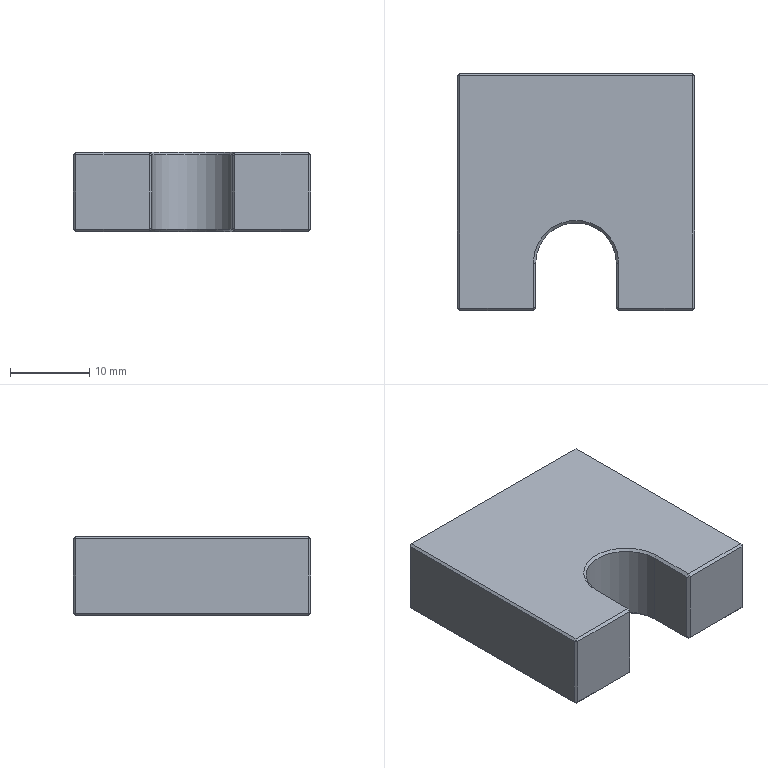Part | SolidWorks | features Chamfer 2, Extrusion 1, HoleWzd 1, ICE 1 | 1 solid | 52 faces | box 30 x 30 x 10 mm | volume 7510 mm3 | plane 41 | cone 6 | cylinder 5 | commonest cylinder face diameters 4.2 x4 10.2 x1
STEP:
#1=CARTESIAN_POINT('',(10.,-1.,2.9));
#2=VERTEX_POINT('',#1);
#3=CARTESIAN_POINT('',(10.,-1.,7.1));
#4=VERTEX_POINT('',#3);
#5=CARTESIAN_POINT('',(10.,-1.,5.));
#6=DIRECTION('',(0.,1.,0.));
#7=DIRECTION('',(0.,0.,1.));
#8=AXIS2_PLACEMENT_3D('',#5,#6,#7);
#9=CIRCLE('',#8,2.1);
#10=EDGE_CURVE('',#2,#4,#9,.T.);
#11=ORIENTED_EDGE('',*,*,#10,.F.);
#12=CARTESIAN_POINT('',(10.,15.,2.9));
#13=VERTEX_POINT('',#12);
#14=CARTESIAN_POINT('',(10.,15.,2.9));
#15=DIRECTION('',(0.,1.,0.));
#16=VECTOR('',#15,1000.);
#17=LINE('',#14,#16);
#18=EDGE_CURVE('',#2,#13,#17,.T.);
#19=ORIENTED_EDGE('',*,*,#18,.T.);
#20=CARTESIAN_POINT('',(10.,15.,7.1));
#21=VERTEX_POINT('',#20);
#22=CARTESIAN_POINT('',(10.,15.,5.));
#23=DIRECTION('',(0.,1.,0.));
#24=DIRECTION('',(0.,0.,1.));
#25=AXIS2_PLACEMENT_3D('',#22,#23,#24);
#26=CIRCLE('',#25,2.1);
#27=EDGE_CURVE('',#13,#21,#26,.T.);
#28=ORIENTED_EDGE('',*,*,#27,.T.);
#29=CARTESIAN_POINT('',(10.,15.,7.1));
#30=DIRECTION('',(0.,1.,0.));
#31=VECTOR('',#30,1000.);
#32=LINE('',#29,#31);
#33=EDGE_CURVE('',#4,#21,#32,.T.);
#34=ORIENTED_EDGE('',*,*,#33,.F.);
#35=EDGE_LOOP('',(#11,#19,#28,#34));
#36=FACE_OUTER_BOUND('',#35,.T.);
#37=CARTESIAN_POINT('',(10.,15.,5.));
#38=DIRECTION('',(0.,1.,0.));
#39=DIRECTION('',(0.,0.,1.));
#40=AXIS2_PLACEMENT_3D('',#37,#38,#39);
#41=CYLINDRICAL_SURFACE('',#40,2.1);
#42=ADVANCED_FACE('',(#36),#41,.F.);
#43=CARTESIAN_POINT('',(10.,-2.262,5.));
#44=VERTEX_POINT('',#43);
#45=CARTESIAN_POINT('',(10.,-1.,7.1));
#46=DIRECTION('',(0.,0.515,0.8572));
#47=VECTOR('',#46,1000.);
#48=LINE('',#45,#47);
#49=EDGE_CURVE('',#44,#4,#48,.T.);
#50=ORIENTED_EDGE('',*,*,#49,.F.);
#51=CARTESIAN_POINT('',(10.,-1.,2.9));
#52=DIRECTION('',(0.,0.515,-0.8572));
#53=VECTOR('',#52,1000.);
#54=LINE('',#51,#53);
#55=EDGE_CURVE('',#44,#2,#54,.T.);
#56=ORIENTED_EDGE('',*,*,#55,.T.);
#57=ORIENTED_EDGE('',*,*,#10,.T.);
#58=EDGE_LOOP('',(#50,#56,#57));
#59=FACE_OUTER_BOUND('',#58,.T.);
#60=CARTESIAN_POINT('',(10.,-1.,5.));
#61=DIRECTION('',(0.,1.,0.));
#62=DIRECTION('',(0.,0.,1.));
#63=AXIS2_PLACEMENT_3D('',#60,#61,#62);
#64=CONICAL_SURFACE('',#63,2.1,1.03);
#65=ADVANCED_FACE('',(#59),#64,.F.);
#66=CARTESIAN_POINT('',(-10.,-1.,2.9));
#67=VERTEX_POINT('',#66);
#68=CARTESIAN_POINT('',(-10.,-1.,7.1));
#69=VERTEX_POINT('',#68);
#70=CARTESIAN_POINT('',(-10.,-1.,5.));
#71=DIRECTION('',(0.,1.,0.));
#72=DIRECTION('',(0.,0.,1.));
#73=AXIS2_PLACEMENT_3D('',#70,#71,#72);
#74=CIRCLE('',#73,2.1);
#75=EDGE_CURVE('',#67,#69,#74,.T.);
#76=ORIENTED_EDGE('',*,*,#75,.F.);
#77=CARTESIAN_POINT('',(-10.,15.,2.9));
#78=VERTEX_POINT('',#77);
#79=CARTESIAN_POINT('',(-10.,15.,2.9));
#80=DIRECTION('',(0.,1.,0.));
#81=VECTOR('',#80,1000.);
#82=LINE('',#79,#81);
#83=EDGE_CURVE('',#67,#78,#82,.T.);
#84=ORIENTED_EDGE('',*,*,#83,.T.);
#85=CARTESIAN_POINT('',(-10.,15.,7.1));
#86=VERTEX_POINT('',#85);
#87=CARTESIAN_POINT('',(-10.,15.,5.));
#88=DIRECTION('',(0.,1.,0.));
#89=DIRECTION('',(0.,0.,1.));
#90=AXIS2_PLACEMENT_3D('',#87,#88,#89);
#91=CIRCLE('',#90,2.1);
#92=EDGE_CURVE('',#78,#86,#91,.T.);
#93=ORIENTED_EDGE('',*,*,#92,.T.);
#94=CARTESIAN_POINT('',(-10.,15.,7.1));
#95=DIRECTION('',(0.,1.,0.));
#96=VECTOR('',#95,1000.);
#97=LINE('',#94,#96);
#98=EDGE_CURVE('',#69,#86,#97,.T.);
#99=ORIENTED_EDGE('',*,*,#98,.F.);
#100=EDGE_LOOP('',(#76,#84,#93,#99));
#101=FACE_OUTER_BOUND('',#100,.T.);
#102=CARTESIAN_POINT('',(-10.,15.,5.));
#103=DIRECTION('',(0.,1.,0.));
#104=DIRECTION('',(0.,0.,1.));
#105=AXIS2_PLACEMENT_3D('',#102,#103,#104);
#106=CYLINDRICAL_SURFACE('',#105,2.1);
#107=ADVANCED_FACE('',(#101),#106,.F.);
#108=CARTESIAN_POINT('',(-10.,-2.262,5.));
#109=VERTEX_POINT('',#108);
#110=CARTESIAN_POINT('',(-10.,-1.,7.1));
#111=DIRECTION('',(0.,0.515,0.8572));
#112=VECTOR('',#111,1000.);
#113=LINE('',#110,#112);
#114=EDGE_CURVE('',#109,#69,#113,.T.);
#115=ORIENTED_EDGE('',*,*,#114,.F.);
#116=CARTESIAN_POINT('',(-10.,-1.,2.9));
#117=DIRECTION('',(0.,0.515,-0.8572));
#118=VECTOR('',#117,1000.);
#119=LINE('',#116,#118);
#120=EDGE_CURVE('',#109,#67,#119,.T.);
#121=ORIENTED_EDGE('',*,*,#120,.T.);
#122=ORIENTED_EDGE('',*,*,#75,.T.);
#123=EDGE_LOOP('',(#115,#121,#122));
#124=FACE_OUTER_BOUND('',#123,.T.);
#125=CARTESIAN_POINT('',(-10.,-1.,5.));
#126=DIRECTION('',(0.,1.,0.));
#127=DIRECTION('',(0.,0.,1.));
#128=AXIS2_PLACEMENT_3D('',#125,#126,#127);
#129=CONICAL_SURFACE('',#128,2.1,1.03);
#130=ADVANCED_FACE('',(#124),#129,.F.);
#131=CARTESIAN_POINT('',(-14.7,-15.,0.3));
#132=VERTEX_POINT('',#131);
#133=CARTESIAN_POINT('',(-5.4,-15.,0.3));
#134=VERTEX_POINT('',#133);
#135=CARTESIAN_POINT('',(-15.,-15.,0.3));
#136=DIRECTION('',(1.,0.,0.));
#137=VECTOR('',#136,1000.);
#138=LINE('',#135,#137);
#139=EDGE_CURVE('',#132,#134,#138,.T.);
#140=ORIENTED_EDGE('',*,*,#139,.T.);
#141=CARTESIAN_POINT('',(-5.4,-15.,9.7));
#142=VERTEX_POINT('',#141);
#143=CARTESIAN_POINT('',(-5.4,-15.,10.));
#144=DIRECTION('',(0.,0.,1.));
#145=VECTOR('',#144,1000.);
#146=LINE('',#143,#145);
#147=EDGE_CURVE('',#134,#142,#146,.T.);
#148=ORIENTED_EDGE('',*,*,#147,.T.);
#149=CARTESIAN_POINT('',(-14.7,-15.,9.7));
#150=VERTEX_POINT('',#149);
#151=CARTESIAN_POINT('',(-15.,-15.,9.7));
#152=DIRECTION('',(-1.,0.,0.));
#153=VECTOR('',#152,1000.);
#154=LINE('',#151,#153);
#155=EDGE_CURVE('',#142,#150,#154,.T.);
#156=ORIENTED_EDGE('',*,*,#155,.T.);
#157=CARTESIAN_POINT('',(-14.7,-15.,10.));
#158=DIRECTION('',(0.,0.,-1.));
#159=VECTOR('',#158,1000.);
#160=LINE('',#157,#159);
#161=EDGE_CURVE('',#150,#132,#160,.T.);
#162=ORIENTED_EDGE('',*,*,#161,.T.);
#163=EDGE_LOOP('',(#140,#148,#156,#162));
#164=FACE_OUTER_BOUND('',#163,.T.);
#165=CARTESIAN_POINT('',(-15.,-15.,10.));
#166=DIRECTION('',(0.,1.,0.));
#167=DIRECTION('',(0.,0.,1.));
#168=AXIS2_PLACEMENT_3D('',#165,#166,#167);
#169=PLANE('',#168);
#170=ADVANCED_FACE('',(#164),#169,.F.);
#171=ORIENTED_EDGE('',*,*,#155,.F.);
#172=CARTESIAN_POINT('',(-5.4,-14.7,10.));
#173=VERTEX_POINT('',#172);
#174=CARTESIAN_POINT('',(-5.4,-14.7,10.));
#175=DIRECTION('',(0.,0.7071,0.7071));
#176=VECTOR('',#175,1000.);
#177=LINE('',#174,#176);
#178=EDGE_CURVE('',#142,#173,#177,.T.);
#179=ORIENTED_EDGE('',*,*,#178,.T.);
#180=CARTESIAN_POINT('',(-14.7,-14.7,10.));
#181=VERTEX_POINT('',#180);
#182=CARTESIAN_POINT('',(15.,-14.7,10.));
#183=DIRECTION('',(1.,0.,0.));
#184=VECTOR('',#183,1000.);
#185=LINE('',#182,#184);
#186=EDGE_CURVE('',#181,#173,#185,.T.);
#187=ORIENTED_EDGE('',*,*,#186,.F.);
#188=CARTESIAN_POINT('',(-14.7,-14.7,10.));
#189=DIRECTION('',(0.,-0.7071,-0.7071));
#190=VECTOR('',#189,1000.);
#191=LINE('',#188,#190);
#192=EDGE_CURVE('',#181,#150,#191,.T.);
#193=ORIENTED_EDGE('',*,*,#192,.T.);
#194=EDGE_LOOP('',(#171,#179,#187,#193));
#195=FACE_OUTER_BOUND('',#194,.T.);
#196=CARTESIAN_POINT('',(0.,-14.7,10.));
#197=DIRECTION('',(0.,-0.7071,0.7071));
#198=DIRECTION('',(-1.,0.,0.));
#199=AXIS2_PLACEMENT_3D('',#196,#197,#198);
#200=PLANE('',#199);
#201=ADVANCED_FACE('',(#195),#200,.T.);
#202=CARTESIAN_POINT('',(-5.4,-14.7,0.));
#203=VERTEX_POINT('',#202);
#204=CARTESIAN_POINT('',(-14.7,-14.7,0.));
#205=VERTEX_POINT('',#204);
#206=CARTESIAN_POINT('',(0.,-14.7,0.));
#207=DIRECTION('',(-1.,0.,0.));
#208=VECTOR('',#207,1000.);
#209=LINE('',#206,#208);
#210=EDGE_CURVE('',#203,#205,#209,.T.);
#211=ORIENTED_EDGE('',*,*,#210,.F.);
#212=CARTESIAN_POINT('',(-5.4,-15.,0.3));
#213=DIRECTION('',(0.,-0.7071,0.7071));
#214=VECTOR('',#213,1000.);
#215=LINE('',#212,#214);
#216=EDGE_CURVE('',#203,#134,#215,.T.);
#217=ORIENTED_EDGE('',*,*,#216,.T.);
#218=ORIENTED_EDGE('',*,*,#139,.F.);
#219=CARTESIAN_POINT('',(-14.7,-14.85,0.15));
#220=DIRECTION('',(0.,0.7071,-0.7071));
#221=VECTOR('',#220,1000.);
#222=LINE('',#219,#221);
#223=EDGE_CURVE('',#132,#205,#222,.T.);
#224=ORIENTED_EDGE('',*,*,#223,.T.);
#225=EDGE_LOOP('',(#211,#217,#218,#224));
#226=FACE_OUTER_BOUND('',#225,.T.);
#227=CARTESIAN_POINT('',(-15.,-15.,0.3));
#228=DIRECTION('',(0.,0.7071,0.7071));
#229=DIRECTION('',(1.,0.,0.));
#230=AXIS2_PLACEMENT_3D('',#227,#228,#229);
#231=PLANE('',#230);
#232=ADVANCED_FACE('',(#226),#231,.F.);
#233=CARTESIAN_POINT('',(15.,14.7,9.7));
#234=VERTEX_POINT('',#233);
#235=CARTESIAN_POINT('',(15.,-14.7,9.7));
#236=VERTEX_POINT('',#235);
#237=CARTESIAN_POINT('',(15.,-15.,9.7));
#238=DIRECTION('',(0.,-1.,0.));
#239=VECTOR('',#238,1000.);
#240=LINE('',#237,#239);
#241=EDGE_CURVE('',#234,#236,#240,.T.);
#242=ORIENTED_EDGE('',*,*,#241,.T.);
#243=CARTESIAN_POINT('',(15.,-14.7,0.3));
#244=VERTEX_POINT('',#243);
#245=CARTESIAN_POINT('',(15.,-14.7,10.));
#246=DIRECTION('',(0.,0.,-1.));
#247=VECTOR('',#246,1000.);
#248=LINE('',#245,#247);
#249=EDGE_CURVE('',#236,#244,#248,.T.);
#250=ORIENTED_EDGE('',*,*,#249,.T.);
#251=CARTESIAN_POINT('',(15.,14.7,0.3));
#252=VERTEX_POINT('',#251);
#253=CARTESIAN_POINT('',(15.,15.,0.3));
#254=DIRECTION('',(0.,1.,0.));
#255=VECTOR('',#254,1000.);
#256=LINE('',#253,#255);
#257=EDGE_CURVE('',#244,#252,#256,.T.);
#258=ORIENTED_EDGE('',*,*,#257,.T.);
#259=CARTESIAN_POINT('',(15.,14.7,10.));
#260=DIRECTION('',(0.,0.,1.));
#261=VECTOR('',#260,1000.);
#262=LINE('',#259,#261);
#263=EDGE_CURVE('',#252,#234,#262,.T.);
#264=ORIENTED_EDGE('',*,*,#263,.T.);
#265=EDGE_LOOP('',(#242,#250,#258,#264));
#266=FACE_OUTER_BOUND('',#265,.T.);
#267=CARTESIAN_POINT('',(15.,15.,10.));
#268=DIRECTION('',(-1.,0.,0.));
#269=DIRECTION('',(0.,-1.,0.));
#270=AXIS2_PLACEMENT_3D('',#267,#268,#269);
#271=PLANE('',#270);
#272=ADVANCED_FACE('',(#266),#271,.F.);
#273=CARTESIAN_POINT('',(-14.7,15.,0.3));
#274=VERTEX_POINT('',#273);
#275=CARTESIAN_POINT('',(-14.7,15.,9.7));
#276=VERTEX_POINT('',#275);
#277=CARTESIAN_POINT('',(-14.7,15.,10.));
#278=DIRECTION('',(0.,0.,1.));
#279=VECTOR('',#278,1000.);
#280=LINE('',#277,#279);
#281=EDGE_CURVE('',#274,#276,#280,.T.);
#282=ORIENTED_EDGE('',*,*,#281,.T.);
#283=CARTESIAN_POINT('',(14.7,15.,9.7));
#284=VERTEX_POINT('',#283);
#285=CARTESIAN_POINT('',(15.,15.,9.7));
#286=DIRECTION('',(1.,0.,0.));
#287=VECTOR('',#286,1000.);
#288=LINE('',#285,#287);
#289=EDGE_CURVE('',#276,#284,#288,.T.);
#290=ORIENTED_EDGE('',*,*,#289,.T.);
#291=CARTESIAN_POINT('',(14.7,15.,0.3));
#292=VERTEX_POINT('',#291);
#293=CARTESIAN_POINT('',(14.7,15.,10.));
#294=DIRECTION('',(0.,0.,-1.));
#295=VECTOR('',#294,1000.);
#296=LINE('',#293,#295);
#297=EDGE_CURVE('',#284,#292,#296,.T.);
#298=ORIENTED_EDGE('',*,*,#297,.T.);
#299=CARTESIAN_POINT('',(-15.,15.,0.3));
#300=DIRECTION('',(-1.,0.,0.));
#301=VECTOR('',#300,1000.);
#302=LINE('',#299,#301);
#303=EDGE_CURVE('',#292,#274,#302,.T.);
#304=ORIENTED_EDGE('',*,*,#303,.T.);
#305=EDGE_LOOP('',(#282,#290,#298,#304));
#306=FACE_OUTER_BOUND('',#305,.T.);
#307=CARTESIAN_POINT('',(10.,15.,5.));
#308=DIRECTION('',(0.,1.,0.));
#309=DIRECTION('',(0.,0.,1.));
#310=AXIS2_PLACEMENT_3D('',#307,#308,#309);
#311=CIRCLE('',#310,2.1);
#312=EDGE_CURVE('',#21,#13,#311,.T.);
#313=ORIENTED_EDGE('',*,*,#312,.F.);
#314=ORIENTED_EDGE('',*,*,#27,.F.);
#315=EDGE_LOOP('',(#313,#314));
#316=FACE_BOUND('',#315,.T.);
#317=CARTESIAN_POINT('',(-10.,15.,5.));
#318=DIRECTION('',(0.,1.,0.));
#319=DIRECTION('',(0.,0.,1.));
#320=AXIS2_PLACEMENT_3D('',#317,#318,#319);
#321=CIRCLE('',#320,2.1);
#322=EDGE_CURVE('',#86,#78,#321,.T.);
#323=ORIENTED_EDGE('',*,*,#322,.F.);
#324=ORIENTED_EDGE('',*,*,#92,.F.);
#325=EDGE_LOOP('',(#323,#324));
#326=FACE_BOUND('',#325,.T.);
#327=CARTESIAN_POINT('',(-15.,15.,10.));
#328=DIRECTION('',(0.,-1.,0.));
#329=DIRECTION('',(0.,0.,-1.));
#330=AXIS2_PLACEMENT_3D('',#327,#328,#329);
#331=PLANE('',#330);
#332=ADVANCED_FACE('',(#306,#316,#326),#331,.F.);
#333=CARTESIAN_POINT('',(-15.,-14.7,9.7));
#334=VERTEX_POINT('',#333);
#335=CARTESIAN_POINT('',(-15.,14.7,9.7));
#336=VERTEX_POINT('',#335);
#337=CARTESIAN_POINT('',(-15.,15.,9.7));
#338=DIRECTION('',(0.,1.,0.));
#339=VECTOR('',#338,1000.);
#340=LINE('',#337,#339);
#341=EDGE_CURVE('',#334,#336,#340,.T.);
#342=ORIENTED_EDGE('',*,*,#341,.T.);
#343=CARTESIAN_POINT('',(-15.,14.7,0.3));
#344=VERTEX_POINT('',#343);
#345=CARTESIAN_POINT('',(-15.,14.7,10.));
#346=DIRECTION('',(0.,0.,-1.));
#347=VECTOR('',#346,1000.);
#348=LINE('',#345,#347);
#349=EDGE_CURVE('',#336,#344,#348,.T.);
#350=ORIENTED_EDGE('',*,*,#349,.T.);
#351=CARTESIAN_POINT('',(-15.,-14.7,0.3));
#352=VERTEX_POINT('',#351);
#353=CARTESIAN_POINT('',(-15.,15.,0.3));
#354=DIRECTION('',(0.,-1.,0.));
#355=VECTOR('',#354,1000.);
#356=LINE('',#353,#355);
#357=EDGE_CURVE('',#344,#352,#356,.T.);
#358=ORIENTED_EDGE('',*,*,#357,.T.);
#359=CARTESIAN_POINT('',(-15.,-14.7,10.));
#360=DIRECTION('',(0.,0.,1.));
#361=VECTOR('',#360,1000.);
#362=LINE('',#359,#361);
#363=EDGE_CURVE('',#352,#334,#362,.T.);
#364=ORIENTED_EDGE('',*,*,#363,.T.);
#365=EDGE_LOOP('',(#342,#350,#358,#364));
#366=FACE_OUTER_BOUND('',#365,.T.);
#367=CARTESIAN_POINT('',(-15.,15.,10.));
#368=DIRECTION('',(1.,0.,0.));
#369=DIRECTION('',(0.,1.,0.));
#370=AXIS2_PLACEMENT_3D('',#367,#368,#369);
#371=PLANE('',#370);
#372=ADVANCED_FACE('',(#366),#371,.F.);
#373=CARTESIAN_POINT('',(14.7,-15.,9.7));
#374=VERTEX_POINT('',#373);
#375=CARTESIAN_POINT('',(5.4,-15.,9.7));
#376=VERTEX_POINT('',#375);
#377=CARTESIAN_POINT('',(-15.,-15.,9.7));
#378=DIRECTION('',(-1.,0.,0.));
#379=VECTOR('',#378,1000.);
#380=LINE('',#377,#379);
#381=EDGE_CURVE('',#374,#376,#380,.T.);
#382=ORIENTED_EDGE('',*,*,#381,.T.);
#383=CARTESIAN_POINT('',(5.4,-15.,0.3));
#384=VERTEX_POINT('',#383);
#385=CARTESIAN_POINT('',(5.4,-15.,10.));
#386=DIRECTION('',(0.,0.,-1.));
#387=VECTOR('',#386,1000.);
#388=LINE('',#385,#387);
#389=EDGE_CURVE('',#376,#384,#388,.T.);
#390=ORIENTED_EDGE('',*,*,#389,.T.);
#391=CARTESIAN_POINT('',(14.7,-15.,0.3));
#392=VERTEX_POINT('',#391);
#393=CARTESIAN_POINT('',(-15.,-15.,0.3));
#394=DIRECTION('',(1.,0.,0.));
#395=VECTOR('',#394,1000.);
#396=LINE('',#393,#395);
#397=EDGE_CURVE('',#384,#392,#396,.T.);
#398=ORIENTED_EDGE('',*,*,#397,.T.);
#399=CARTESIAN_POINT('',(14.7,-15.,10.));
#400=DIRECTION('',(0.,0.,1.));
#401=VECTOR('',#400,1000.);
#402=LINE('',#399,#401);
#403=EDGE_CURVE('',#392,#374,#402,.T.);
#404=ORIENTED_EDGE('',*,*,#403,.T.);
#405=EDGE_LOOP('',(#382,#390,#398,#404));
#406=FACE_OUTER_BOUND('',#405,.T.);
#407=CARTESIAN_POINT('',(-15.,-15.,10.));
#408=DIRECTION('',(0.,1.,0.));
#409=DIRECTION('',(0.,0.,1.));
#410=AXIS2_PLACEMENT_3D('',#407,#408,#409);
#411=PLANE('',#410);
#412=ADVANCED_FACE('',(#406),#411,.F.);
#413=CARTESIAN_POINT('',(-5.4,-9.,10.));
#414=VERTEX_POINT('',#413);
#415=CARTESIAN_POINT('',(5.4,-9.,10.));
#416=VERTEX_POINT('',#415);
#417=CARTESIAN_POINT('',(0.,-9.,10.));
#418=DIRECTION('',(0.,0.,-1.));
#419=DIRECTION('',(1.,0.,0.));
#420=AXIS2_PLACEMENT_3D('',#417,#418,#419);
#421=CIRCLE('',#420,5.4);
#422=EDGE_CURVE('',#414,#416,#421,.T.);
#423=ORIENTED_EDGE('',*,*,#422,.T.);
#424=CARTESIAN_POINT('',(5.4,-14.7,10.));
#425=VERTEX_POINT('',#424);
#426=CARTESIAN_POINT('',(5.4,-14.7,10.));
#427=DIRECTION('',(0.,-1.,0.));
#428=VECTOR('',#427,1000.);
#429=LINE('',#426,#428);
#430=EDGE_CURVE('',#416,#425,#429,.T.);
#431=ORIENTED_EDGE('',*,*,#430,.T.);
#432=CARTESIAN_POINT('',(14.7,-14.7,10.));
#433=VERTEX_POINT('',#432);
#434=CARTESIAN_POINT('',(15.,-14.7,10.));
#435=DIRECTION('',(1.,0.,0.));
#436=VECTOR('',#435,1000.);
#437=LINE('',#434,#436);
#438=EDGE_CURVE('',#425,#433,#437,.T.);
#439=ORIENTED_EDGE('',*,*,#438,.T.);
#440=CARTESIAN_POINT('',(14.7,14.7,10.));
#441=VERTEX_POINT('',#440);
#442=CARTESIAN_POINT('',(14.7,15.,10.));
#443=DIRECTION('',(0.,1.,0.));
#444=VECTOR('',#443,1000.);
#445=LINE('',#442,#444);
#446=EDGE_CURVE('',#433,#441,#445,.T.);
#447=ORIENTED_EDGE('',*,*,#446,.T.);
#448=CARTESIAN_POINT('',(-14.7,14.7,10.));
#449=VERTEX_POINT('',#448);
#450=CARTESIAN_POINT('',(-15.,14.7,10.));
#451=DIRECTION('',(-1.,0.,0.));
#452=VECTOR('',#451,1000.);
#453=LINE('',#450,#452);
#454=EDGE_CURVE('',#441,#449,#453,.T.);
#455=ORIENTED_EDGE('',*,*,#454,.T.);
#456=CARTESIAN_POINT('',(-14.7,-15.,10.));
#457=DIRECTION('',(0.,-1.,0.));
#458=VECTOR('',#457,1000.);
#459=LINE('',#456,#458);
#460=EDGE_CURVE('',#449,#181,#459,.T.);
#461=ORIENTED_EDGE('',*,*,#460,.T.);
#462=ORIENTED_EDGE('',*,*,#186,.T.);
#463=CARTESIAN_POINT('',(-5.4,-9.,10.));
#464=DIRECTION('',(0.,1.,0.));
#465=VECTOR('',#464,1000.);
#466=LINE('',#463,#465);
#467=EDGE_CURVE('',#173,#414,#466,.T.);
#468=ORIENTED_EDGE('',*,*,#467,.T.);
#469=EDGE_LOOP('',(#423,#431,#439,#447,#455,#461,#462,#468));
#470=FACE_OUTER_BOUND('',#469,.T.);
#471=CARTESIAN_POINT('',(0.,0.,10.));
#472=DIRECTION('',(0.,0.,1.));
#473=DIRECTION('',(1.,0.,0.));
#474=AXIS2_PLACEMENT_3D('',#471,#472,#473);
#475=PLANE('',#474);
#476=ADVANCED_FACE('',(#470),#475,.T.);
#477=CARTESIAN_POINT('',(14.7,-14.7,0.));
#478=VERTEX_POINT('',#477);
#479=CARTESIAN_POINT('',(5.4,-14.7,0.));
#480=VERTEX_POINT('',#479);
#481=CARTESIAN_POINT('',(0.,-14.7,0.));
#482=DIRECTION('',(-1.,0.,0.));
#483=VECTOR('',#482,1000.);
#484=LINE('',#481,#483);
#485=EDGE_CURVE('',#478,#480,#484,.T.);
#486=ORIENTED_EDGE('',*,*,#485,.T.);
#487=CARTESIAN_POINT('',(5.4,-9.,0.));
#488=VERTEX_POINT('',#487);
#489=CARTESIAN_POINT('',(5.4,0.,0.));
#490=DIRECTION('',(0.,1.,0.));
#491=VECTOR('',#490,1000.);
#492=LINE('',#489,#491);
#493=EDGE_CURVE('',#480,#488,#492,.T.);
#494=ORIENTED_EDGE('',*,*,#493,.T.);
#495=CARTESIAN_POINT('',(-5.4,-9.,0.));
#496=VERTEX_POINT('',#495);
#497=CARTESIAN_POINT('',(0.,-9.,0.));
#498=DIRECTION('',(0.,0.,1.));
#499=DIRECTION('',(1.,0.,0.));
#500=AXIS2_PLACEMENT_3D('',#497,#498,#499);
#501=CIRCLE('',#500,5.4);
#502=EDGE_CURVE('',#488,#496,#501,.T.);
#503=ORIENTED_EDGE('',*,*,#502,.T.);
#504=CARTESIAN_POINT('',(-5.4,0.,0.));
#505=DIRECTION('',(0.,-1.,0.));
#506=VECTOR('',#505,1000.);
#507=LINE('',#504,#506);
#508=EDGE_CURVE('',#496,#203,#507,.T.);
#509=ORIENTED_EDGE('',*,*,#508,.T.);
#510=ORIENTED_EDGE('',*,*,#210,.T.);
#511=CARTESIAN_POINT('',(-14.7,14.7,0.));
#512=VERTEX_POINT('',#511);
#513=CARTESIAN_POINT('',(-14.7,0.,0.));
#514=DIRECTION('',(0.,1.,0.));
#515=VECTOR('',#514,1000.);
#516=LINE('',#513,#515);
#517=EDGE_CURVE('',#205,#512,#516,.T.);
#518=ORIENTED_EDGE('',*,*,#517,.T.);
#519=CARTESIAN_POINT('',(14.7,14.7,0.));
#520=VERTEX_POINT('',#519);
#521=CARTESIAN_POINT('',(0.,14.7,0.));
#522=DIRECTION('',(1.,0.,0.));
#523=VECTOR('',#522,1000.);
#524=LINE('',#521,#523);
#525=EDGE_CURVE('',#512,#520,#524,.T.);
#526=ORIENTED_EDGE('',*,*,#525,.T.);
#527=CARTESIAN_POINT('',(14.7,0.,0.));
#528=DIRECTION('',(0.,-1.,0.));
#529=VECTOR('',#528,1000.);
#530=LINE('',#527,#529);
#531=EDGE_CURVE('',#520,#478,#530,.T.);
#532=ORIENTED_EDGE('',*,*,#531,.T.);
#533=EDGE_LOOP('',(#486,#494,#503,#509,#510,#518,#526,#532));
#534=FACE_OUTER_BOUND('',#533,.T.);
#535=CARTESIAN_POINT('',(0.,0.,0.));
#536=DIRECTION('',(0.,0.,1.));
#537=DIRECTION('',(1.,0.,0.));
#538=AXIS2_PLACEMENT_3D('',#535,#536,#537);
#539=PLANE('',#538);
#540=ADVANCED_FACE('',(#534),#539,.F.);
#541=ORIENTED_EDGE('',*,*,#120,.F.);
#542=ORIENTED_EDGE('',*,*,#114,.T.);
#543=CARTESIAN_POINT('',(-10.,-1.,5.));
#544=DIRECTION('',(0.,1.,0.));
#545=DIRECTION('',(0.,0.,1.));
#546=AXIS2_PLACEMENT_3D('',#543,#544,#545);
#547=CIRCLE('',#546,2.1);
#548=EDGE_CURVE('',#69,#67,#547,.T.);
#549=ORIENTED_EDGE('',*,*,#548,.T.);
#550=EDGE_LOOP('',(#541,#542,#549));
#551=FACE_OUTER_BOUND('',#550,.T.);
#552=CARTESIAN_POINT('',(-10.,-1.,5.));
#553=DIRECTION('',(0.,1.,0.));
#554=DIRECTION('',(0.,0.,1.));
#555=AXIS2_PLACEMENT_3D('',#552,#553,#554);
#556=CONICAL_SURFACE('',#555,2.1,1.03);
#557=ADVANCED_FACE('',(#551),#556,.F.);
#558=ORIENTED_EDGE('',*,*,#83,.F.);
#559=ORIENTED_EDGE('',*,*,#548,.F.);
#560=ORIENTED_EDGE('',*,*,#98,.T.);
#561=ORIENTED_EDGE('',*,*,#322,.T.);
#562=EDGE_LOOP('',(#558,#559,#560,#561));
#563=FACE_OUTER_BOUND('',#562,.T.);
#564=CARTESIAN_POINT('',(-10.,15.,5.));
#565=DIRECTION('',(0.,1.,0.));
#566=DIRECTION('',(0.,0.,1.));
#567=AXIS2_PLACEMENT_3D('',#564,#565,#566);
#568=CYLINDRICAL_SURFACE('',#567,2.1);
#569=ADVANCED_FACE('',(#563),#568,.F.);
#570=ORIENTED_EDGE('',*,*,#55,.F.);
#571=ORIENTED_EDGE('',*,*,#49,.T.);
#572=CARTESIAN_POINT('',(10.,-1.,5.));
#573=DIRECTION('',(0.,1.,0.));
#574=DIRECTION('',(0.,0.,1.));
#575=AXIS2_PLACEMENT_3D('',#572,#573,#574);
#576=CIRCLE('',#575,2.1);
#577=EDGE_CURVE('',#4,#2,#576,.T.);
#578=ORIENTED_EDGE('',*,*,#577,.T.);
#579=EDGE_LOOP('',(#570,#571,#578));
#580=FACE_OUTER_BOUND('',#579,.T.);
#581=CARTESIAN_POINT('',(10.,-1.,5.));
#582=DIRECTION('',(0.,1.,0.));
#583=DIRECTION('',(0.,0.,1.));
#584=AXIS2_PLACEMENT_3D('',#581,#582,#583);
#585=CONICAL_SURFACE('',#584,2.1,1.03);
#586=ADVANCED_FACE('',(#580),#585,.F.);
#587=ORIENTED_EDGE('',*,*,#18,.F.);
#588=ORIENTED_EDGE('',*,*,#577,.F.);
#589=ORIENTED_EDGE('',*,*,#33,.T.);
#590=ORIENTED_EDGE('',*,*,#312,.T.);
#591=EDGE_LOOP('',(#587,#588,#589,#590));
#592=FACE_OUTER_BOUND('',#591,.T.);
#593=CARTESIAN_POINT('',(10.,15.,5.));
#594=DIRECTION('',(0.,1.,0.));
#595=DIRECTION('',(0.,0.,1.));
#596=AXIS2_PLACEMENT_3D('',#593,#594,#595);
#597=CYLINDRICAL_SURFACE('',#596,2.1);
#598=ADVANCED_FACE('',(#592),#597,.F.);
#599=CARTESIAN_POINT('',(-14.7,15.,9.7));
#600=DIRECTION('',(-0.7071,-0.7071,0.));
#601=VECTOR('',#600,1000.);
#602=LINE('',#599,#601);
#603=EDGE_CURVE('',#276,#336,#602,.T.);
#604=ORIENTED_EDGE('',*,*,#603,.F.);
#605=ORIENTED_EDGE('',*,*,#281,.F.);
#606=CARTESIAN_POINT('',(-15.,14.7,0.3));
#607=DIRECTION('',(0.7071,0.7071,0.));
#608=VECTOR('',#607,1000.);
#609=LINE('',#606,#608);
#610=EDGE_CURVE('',#344,#274,#609,.T.);
#611=ORIENTED_EDGE('',*,*,#610,.F.);
#612=ORIENTED_EDGE('',*,*,#349,.F.);
#613=EDGE_LOOP('',(#604,#605,#611,#612));
#614=FACE_OUTER_BOUND('',#613,.T.);
#615=CARTESIAN_POINT('',(-15.,14.7,10.));
#616=DIRECTION('',(0.7071,-0.7071,0.));
#617=DIRECTION('',(0.,0.,-1.));
#618=AXIS2_PLACEMENT_3D('',#615,#616,#617);
#619=PLANE('',#618);
#620=ADVANCED_FACE('',(#614),#619,.F.);
#621=CARTESIAN_POINT('',(-14.7,15.,9.7));
#622=DIRECTION('',(0.,-0.7071,0.7071));
#623=VECTOR('',#622,1000.);
#624=LINE('',#621,#623);
#625=EDGE_CURVE('',#276,#449,#624,.T.);
#626=ORIENTED_EDGE('',*,*,#625,.F.);
#627=ORIENTED_EDGE('',*,*,#603,.T.);
#628=CARTESIAN_POINT('',(-14.85,14.7,9.85));
#629=DIRECTION('',(-0.7071,0.,-0.7071));
#630=VECTOR('',#629,1000.);
#631=LINE('',#628,#630);
#632=EDGE_CURVE('',#449,#336,#631,.T.);
#633=ORIENTED_EDGE('',*,*,#632,.F.);
#634=EDGE_LOOP('',(#626,#627,#633));
#635=FACE_OUTER_BOUND('',#634,.T.);
#636=CARTESIAN_POINT('',(-14.7,15.,9.7));
#637=DIRECTION('',(-0.5774,0.5774,0.5774));
#638=DIRECTION('',(0.7071,0.,0.7071));
#639=AXIS2_PLACEMENT_3D('',#636,#637,#638);
#640=PLANE('',#639);
#641=ADVANCED_FACE('',(#635),#640,.T.);
#642=CARTESIAN_POINT('',(-15.,14.7,0.3));
#643=DIRECTION('',(0.7071,0.,-0.7071));
#644=VECTOR('',#643,1000.);
#645=LINE('',#642,#644);
#646=EDGE_CURVE('',#344,#512,#645,.T.);
#647=ORIENTED_EDGE('',*,*,#646,.F.);
#648=ORIENTED_EDGE('',*,*,#610,.T.);
#649=CARTESIAN_POINT('',(-14.7,14.85,0.15));
#650=DIRECTION('',(0.,0.7071,0.7071));
#651=VECTOR('',#650,1000.);
#652=LINE('',#649,#651);
#653=EDGE_CURVE('',#512,#274,#652,.T.);
#654=ORIENTED_EDGE('',*,*,#653,.F.);
#655=EDGE_LOOP('',(#647,#648,#654));
#656=FACE_OUTER_BOUND('',#655,.T.);
#657=CARTESIAN_POINT('',(-15.,14.7,0.3));
#658=DIRECTION('',(-0.5774,0.5774,-0.5774));
#659=DIRECTION('',(-0.7071,0.,0.7071));
#660=AXIS2_PLACEMENT_3D('',#657,#658,#659);
#661=PLANE('',#660);
#662=ADVANCED_FACE('',(#656),#661,.T.);
#663=ORIENTED_EDGE('',*,*,#632,.T.);
#664=ORIENTED_EDGE('',*,*,#341,.F.);
#665=CARTESIAN_POINT('',(-14.7,-14.7,10.));
#666=DIRECTION('',(-0.7071,0.,-0.7071));
#667=VECTOR('',#666,1000.);
#668=LINE('',#665,#667);
#669=EDGE_CURVE('',#181,#334,#668,.T.);
#670=ORIENTED_EDGE('',*,*,#669,.F.);
#671=ORIENTED_EDGE('',*,*,#460,.F.);
#672=EDGE_LOOP('',(#663,#664,#670,#671));
#673=FACE_OUTER_BOUND('',#672,.T.);
#674=CARTESIAN_POINT('',(-14.7,0.,10.));
#675=DIRECTION('',(-0.7071,0.,0.7071));
#676=DIRECTION('',(0.,1.,0.));
#677=AXIS2_PLACEMENT_3D('',#674,#675,#676);
#678=PLANE('',#677);
#679=ADVANCED_FACE('',(#673),#678,.T.);
#680=ORIENTED_EDGE('',*,*,#625,.T.);
#681=ORIENTED_EDGE('',*,*,#454,.F.);
#682=CARTESIAN_POINT('',(14.7,14.7,10.));
#683=DIRECTION('',(0.,-0.7071,0.7071));
#684=VECTOR('',#683,1000.);
#685=LINE('',#682,#684);
#686=EDGE_CURVE('',#284,#441,#685,.T.);
#687=ORIENTED_EDGE('',*,*,#686,.F.);
#688=ORIENTED_EDGE('',*,*,#289,.F.);
#689=EDGE_LOOP('',(#680,#681,#687,#688));
#690=FACE_OUTER_BOUND('',#689,.T.);
#691=CARTESIAN_POINT('',(0.,14.7,10.));
#692=DIRECTION('',(0.,0.7071,0.7071));
#693=DIRECTION('',(1.,0.,0.));
#694=AXIS2_PLACEMENT_3D('',#691,#692,#693);
#695=PLANE('',#694);
#696=ADVANCED_FACE('',(#690),#695,.T.);
#697=CARTESIAN_POINT('',(14.7,15.,0.3));
#698=DIRECTION('',(0.7071,-0.7071,0.));
#699=VECTOR('',#698,1000.);
#700=LINE('',#697,#699);
#701=EDGE_CURVE('',#292,#252,#700,.T.);
#702=ORIENTED_EDGE('',*,*,#701,.F.);
#703=ORIENTED_EDGE('',*,*,#297,.F.);
#704=CARTESIAN_POINT('',(14.85,14.85,9.7));
#705=DIRECTION('',(-0.7071,0.7071,0.));
#706=VECTOR('',#705,1000.);
#707=LINE('',#704,#706);
#708=EDGE_CURVE('',#234,#284,#707,.T.);
#709=ORIENTED_EDGE('',*,*,#708,.F.);
#710=ORIENTED_EDGE('',*,*,#263,.F.);
#711=EDGE_LOOP('',(#702,#703,#709,#710));
#712=FACE_OUTER_BOUND('',#711,.T.);
#713=CARTESIAN_POINT('',(14.7,15.,10.));
#714=DIRECTION('',(-0.7071,-0.7071,0.));
#715=DIRECTION('',(0.,0.,-1.));
#716=AXIS2_PLACEMENT_3D('',#713,#714,#715);
#717=PLANE('',#716);
#718=ADVANCED_FACE('',(#712),#717,.F.);
#719=ORIENTED_EDGE('',*,*,#653,.T.);
#720=ORIENTED_EDGE('',*,*,#303,.F.);
#721=CARTESIAN_POINT('',(14.7,15.,0.3));
#722=DIRECTION('',(0.,0.7071,0.7071));
#723=VECTOR('',#722,1000.);
#724=LINE('',#721,#723);
#725=EDGE_CURVE('',#520,#292,#724,.T.);
#726=ORIENTED_EDGE('',*,*,#725,.F.);
#727=ORIENTED_EDGE('',*,*,#525,.F.);
#728=EDGE_LOOP('',(#719,#720,#726,#727));
#729=FACE_OUTER_BOUND('',#728,.T.);
#730=CARTESIAN_POINT('',(-15.,15.,0.3));
#731=DIRECTION('',(0.,-0.7071,0.7071));
#732=DIRECTION('',(-1.,0.,0.));
#733=AXIS2_PLACEMENT_3D('',#730,#731,#732);
#734=PLANE('',#733);
#735=ADVANCED_FACE('',(#729),#734,.F.);
#736=ORIENTED_EDGE('',*,*,#646,.T.);
#737=ORIENTED_EDGE('',*,*,#517,.F.);
#738=CARTESIAN_POINT('',(-15.,-14.7,0.3));
#739=DIRECTION('',(0.7071,0.,-0.7071));
#740=VECTOR('',#739,1000.);
#741=LINE('',#738,#740);
#742=EDGE_CURVE('',#352,#205,#741,.T.);
#743=ORIENTED_EDGE('',*,*,#742,.F.);
#744=ORIENTED_EDGE('',*,*,#357,.F.);
#745=EDGE_LOOP('',(#736,#737,#743,#744));
#746=FACE_OUTER_BOUND('',#745,.T.);
#747=CARTESIAN_POINT('',(-15.,15.,0.3));
#748=DIRECTION('',(0.7071,0.,0.7071));
#749=DIRECTION('',(0.,-1.,0.));
#750=AXIS2_PLACEMENT_3D('',#747,#748,#749);
#751=PLANE('',#750);
#752=ADVANCED_FACE('',(#746),#751,.F.);
#753=CARTESIAN_POINT('',(-14.85,-14.85,9.7));
#754=DIRECTION('',(0.7071,-0.7071,0.));
#755=VECTOR('',#754,1000.);
#756=LINE('',#753,#755);
#757=EDGE_CURVE('',#334,#150,#756,.T.);
#758=ORIENTED_EDGE('',*,*,#757,.F.);
#759=ORIENTED_EDGE('',*,*,#363,.F.);
#760=CARTESIAN_POINT('',(-15.,-14.7,0.3));
#761=DIRECTION('',(-0.7071,0.7071,0.));
#762=VECTOR('',#761,1000.);
#763=LINE('',#760,#762);
#764=EDGE_CURVE('',#132,#352,#763,.T.);
#765=ORIENTED_EDGE('',*,*,#764,.F.);
#766=ORIENTED_EDGE('',*,*,#161,.F.);
#767=EDGE_LOOP('',(#758,#759,#765,#766));
#768=FACE_OUTER_BOUND('',#767,.T.);
#769=CARTESIAN_POINT('',(-14.7,-15.,10.));
#770=DIRECTION('',(0.7071,0.7071,0.));
#771=DIRECTION('',(0.,0.,-1.));
#772=AXIS2_PLACEMENT_3D('',#769,#770,#771);
#773=PLANE('',#772);
#774=ADVANCED_FACE('',(#768),#773,.F.);
#775=ORIENTED_EDGE('',*,*,#669,.T.);
#776=ORIENTED_EDGE('',*,*,#757,.T.);
#777=ORIENTED_EDGE('',*,*,#192,.F.);
#778=EDGE_LOOP('',(#775,#776,#777));
#779=FACE_OUTER_BOUND('',#778,.T.);
#780=CARTESIAN_POINT('',(-14.7,-14.7,10.));
#781=DIRECTION('',(-0.5774,-0.5774,0.5774));
#782=DIRECTION('',(0.7071,0.,0.7071));
#783=AXIS2_PLACEMENT_3D('',#780,#781,#782);
#784=PLANE('',#783);
#785=ADVANCED_FACE('',(#779),#784,.T.);
#786=ORIENTED_EDGE('',*,*,#708,.T.);
#787=ORIENTED_EDGE('',*,*,#686,.T.);
#788=CARTESIAN_POINT('',(14.7,14.7,10.));
#789=DIRECTION('',(-0.7071,0.,0.7071));
#790=VECTOR('',#789,1000.);
#791=LINE('',#788,#790);
#792=EDGE_CURVE('',#234,#441,#791,.T.);
#793=ORIENTED_EDGE('',*,*,#792,.F.);
#794=EDGE_LOOP('',(#786,#787,#793));
#795=FACE_OUTER_BOUND('',#794,.T.);
#796=CARTESIAN_POINT('',(14.7,14.7,10.));
#797=DIRECTION('',(0.5774,0.5774,0.5774));
#798=DIRECTION('',(0.7071,0.,-0.7071));
#799=AXIS2_PLACEMENT_3D('',#796,#797,#798);
#800=PLANE('',#799);
#801=ADVANCED_FACE('',(#795),#800,.T.);
#802=ORIENTED_EDGE('',*,*,#725,.T.);
#803=ORIENTED_EDGE('',*,*,#701,.T.);
#804=CARTESIAN_POINT('',(14.85,14.7,0.15));
#805=DIRECTION('',(0.7071,0.,0.7071));
#806=VECTOR('',#805,1000.);
#807=LINE('',#804,#806);
#808=EDGE_CURVE('',#520,#252,#807,.T.);
#809=ORIENTED_EDGE('',*,*,#808,.F.);
#810=EDGE_LOOP('',(#802,#803,#809));
#811=FACE_OUTER_BOUND('',#810,.T.);
#812=CARTESIAN_POINT('',(14.7,15.,0.3));
#813=DIRECTION('',(0.5774,0.5774,-0.5774));
#814=DIRECTION('',(-0.7071,0.,-0.7071));
#815=AXIS2_PLACEMENT_3D('',#812,#813,#814);
#816=PLANE('',#815);
#817=ADVANCED_FACE('',(#811),#816,.T.);
#818=ORIENTED_EDGE('',*,*,#764,.T.);
#819=ORIENTED_EDGE('',*,*,#742,.T.);
#820=ORIENTED_EDGE('',*,*,#223,.F.);
#821=EDGE_LOOP('',(#818,#819,#820));
#822=FACE_OUTER_BOUND('',#821,.T.);
#823=CARTESIAN_POINT('',(-15.,-14.7,0.3));
#824=DIRECTION('',(-0.5774,-0.5774,-0.5774));
#825=DIRECTION('',(-0.7071,0.,0.7071));
#826=AXIS2_PLACEMENT_3D('',#823,#824,#825);
#827=PLANE('',#826);
#828=ADVANCED_FACE('',(#822),#827,.T.);
#829=ORIENTED_EDGE('',*,*,#438,.F.);
#830=CARTESIAN_POINT('',(5.4,-15.,9.7));
#831=DIRECTION('',(0.,-0.7071,-0.7071));
#832=VECTOR('',#831,1000.);
#833=LINE('',#830,#832);
#834=EDGE_CURVE('',#425,#376,#833,.T.);
#835=ORIENTED_EDGE('',*,*,#834,.T.);
#836=ORIENTED_EDGE('',*,*,#381,.F.);
#837=CARTESIAN_POINT('',(14.7,-15.,9.7));
#838=DIRECTION('',(0.,-0.7071,-0.7071));
#839=VECTOR('',#838,1000.);
#840=LINE('',#837,#839);
#841=EDGE_CURVE('',#433,#374,#840,.T.);
#842=ORIENTED_EDGE('',*,*,#841,.F.);
#843=EDGE_LOOP('',(#829,#835,#836,#842));
#844=FACE_OUTER_BOUND('',#843,.T.);
#845=CARTESIAN_POINT('',(0.,-14.7,10.));
#846=DIRECTION('',(0.,-0.7071,0.7071));
#847=DIRECTION('',(-1.,0.,0.));
#848=AXIS2_PLACEMENT_3D('',#845,#846,#847);
#849=PLANE('',#848);
#850=ADVANCED_FACE('',(#844),#849,.T.);
#851=ORIENTED_EDGE('',*,*,#792,.T.);
#852=ORIENTED_EDGE('',*,*,#446,.F.);
#853=CARTESIAN_POINT('',(14.85,-14.7,9.85));
#854=DIRECTION('',(-0.7071,0.,0.7071));
#855=VECTOR('',#854,1000.);
#856=LINE('',#853,#855);
#857=EDGE_CURVE('',#236,#433,#856,.T.);
#858=ORIENTED_EDGE('',*,*,#857,.F.);
#859=ORIENTED_EDGE('',*,*,#241,.F.);
#860=EDGE_LOOP('',(#851,#852,#858,#859));
#861=FACE_OUTER_BOUND('',#860,.T.);
#862=CARTESIAN_POINT('',(14.7,0.,10.));
#863=DIRECTION('',(0.7071,0.,0.7071));
#864=DIRECTION('',(0.,-1.,0.));
#865=AXIS2_PLACEMENT_3D('',#862,#863,#864);
#866=PLANE('',#865);
#867=ADVANCED_FACE('',(#861),#866,.T.);
#868=ORIENTED_EDGE('',*,*,#808,.T.);
#869=ORIENTED_EDGE('',*,*,#257,.F.);
#870=CARTESIAN_POINT('',(15.,-14.7,0.3));
#871=DIRECTION('',(0.7071,0.,0.7071));
#872=VECTOR('',#871,1000.);
#873=LINE('',#870,#872);
#874=EDGE_CURVE('',#478,#244,#873,.T.);
#875=ORIENTED_EDGE('',*,*,#874,.F.);
#876=ORIENTED_EDGE('',*,*,#531,.F.);
#877=EDGE_LOOP('',(#868,#869,#875,#876));
#878=FACE_OUTER_BOUND('',#877,.T.);
#879=CARTESIAN_POINT('',(15.,15.,0.3));
#880=DIRECTION('',(-0.7071,0.,0.7071));
#881=DIRECTION('',(0.,1.,0.));
#882=AXIS2_PLACEMENT_3D('',#879,#880,#881);
#883=PLANE('',#882);
#884=ADVANCED_FACE('',(#878),#883,.F.);
#885=ORIENTED_EDGE('',*,*,#397,.F.);
#886=CARTESIAN_POINT('',(5.4,-14.7,0.));
#887=DIRECTION('',(0.,0.7071,-0.7071));
#888=VECTOR('',#887,1000.);
#889=LINE('',#886,#888);
#890=EDGE_CURVE('',#384,#480,#889,.T.);
#891=ORIENTED_EDGE('',*,*,#890,.T.);
#892=ORIENTED_EDGE('',*,*,#485,.F.);
#893=CARTESIAN_POINT('',(14.7,-14.85,0.15));
#894=DIRECTION('',(0.,0.7071,-0.7071));
#895=VECTOR('',#894,1000.);
#896=LINE('',#893,#895);
#897=EDGE_CURVE('',#392,#478,#896,.T.);
#898=ORIENTED_EDGE('',*,*,#897,.F.);
#899=EDGE_LOOP('',(#885,#891,#892,#898));
#900=FACE_OUTER_BOUND('',#899,.T.);
#901=CARTESIAN_POINT('',(-15.,-15.,0.3));
#902=DIRECTION('',(0.,0.7071,0.7071));
#903=DIRECTION('',(1.,0.,0.));
#904=AXIS2_PLACEMENT_3D('',#901,#902,#903);
#905=PLANE('',#904);
#906=ADVANCED_FACE('',(#900),#905,.F.);
#907=ORIENTED_EDGE('',*,*,#857,.T.);
#908=ORIENTED_EDGE('',*,*,#841,.T.);
#909=CARTESIAN_POINT('',(14.7,-15.,9.7));
#910=DIRECTION('',(-0.7071,-0.7071,0.));
#911=VECTOR('',#910,1000.);
#912=LINE('',#909,#911);
#913=EDGE_CURVE('',#236,#374,#912,.T.);
#914=ORIENTED_EDGE('',*,*,#913,.F.);
#915=EDGE_LOOP('',(#907,#908,#914));
#916=FACE_OUTER_BOUND('',#915,.T.);
#917=CARTESIAN_POINT('',(14.7,-15.,9.7));
#918=DIRECTION('',(0.5774,-0.5774,0.5774));
#919=DIRECTION('',(0.,-0.7071,-0.7071));
#920=AXIS2_PLACEMENT_3D('',#917,#918,#919);
#921=PLANE('',#920);
#922=ADVANCED_FACE('',(#916),#921,.T.);
#923=ORIENTED_EDGE('',*,*,#897,.T.);
#924=ORIENTED_EDGE('',*,*,#874,.T.);
#925=CARTESIAN_POINT('',(15.,-14.7,0.3));
#926=DIRECTION('',(0.7071,0.7071,0.));
#927=VECTOR('',#926,1000.);
#928=LINE('',#925,#927);
#929=EDGE_CURVE('',#392,#244,#928,.T.);
#930=ORIENTED_EDGE('',*,*,#929,.F.);
#931=EDGE_LOOP('',(#923,#924,#930));
#932=FACE_OUTER_BOUND('',#931,.T.);
#933=CARTESIAN_POINT('',(15.,-14.7,0.3));
#934=DIRECTION('',(0.5774,-0.5774,-0.5774));
#935=DIRECTION('',(0.,0.7071,-0.7071));
#936=AXIS2_PLACEMENT_3D('',#933,#934,#935);
#937=PLANE('',#936);
#938=ADVANCED_FACE('',(#932),#937,.T.);
#939=ORIENTED_EDGE('',*,*,#913,.T.);
#940=ORIENTED_EDGE('',*,*,#403,.F.);
#941=ORIENTED_EDGE('',*,*,#929,.T.);
#942=ORIENTED_EDGE('',*,*,#249,.F.);
#943=EDGE_LOOP('',(#939,#940,#941,#942));
#944=FACE_OUTER_BOUND('',#943,.T.);
#945=CARTESIAN_POINT('',(15.,-14.7,10.));
#946=DIRECTION('',(-0.7071,0.7071,0.));
#947=DIRECTION('',(0.,0.,-1.));
#948=AXIS2_PLACEMENT_3D('',#945,#946,#947);
#949=PLANE('',#948);
#950=ADVANCED_FACE('',(#944),#949,.F.);
#951=CARTESIAN_POINT('',(-5.1,-14.7,0.4243));
#952=VERTEX_POINT('',#951);
#953=CARTESIAN_POINT('',(-5.1,-14.576,0.3));
#954=VERTEX_POINT('',#953);
#955=CARTESIAN_POINT('',(-5.1,-14.488,0.2121));
#956=DIRECTION('',(0.,0.7071,-0.7071));
#957=VECTOR('',#956,1000.);
#958=LINE('',#955,#957);
#959=EDGE_CURVE('',#952,#954,#958,.T.);
#960=ORIENTED_EDGE('',*,*,#959,.T.);
#961=CARTESIAN_POINT('',(-5.1,-9.,0.3));
#962=VERTEX_POINT('',#961);
#963=CARTESIAN_POINT('',(-5.1,-15.,0.3));
#964=DIRECTION('',(0.,1.,0.));
#965=VECTOR('',#964,1000.);
#966=LINE('',#963,#965);
#967=EDGE_CURVE('',#954,#962,#966,.T.);
#968=ORIENTED_EDGE('',*,*,#967,.T.);
#969=CARTESIAN_POINT('',(-5.1,-9.,9.7));
#970=VERTEX_POINT('',#969);
#971=CARTESIAN_POINT('',(-5.1,-9.,0.));
#972=DIRECTION('',(0.,0.,1.));
#973=VECTOR('',#972,1000.);
#974=LINE('',#971,#973);
#975=EDGE_CURVE('',#962,#970,#974,.T.);
#976=ORIENTED_EDGE('',*,*,#975,.T.);
#977=CARTESIAN_POINT('',(-5.1,-14.576,9.7));
#978=VERTEX_POINT('',#977);
#979=CARTESIAN_POINT('',(-5.1,-14.7,9.7));
#980=DIRECTION('',(0.,-1.,0.));
#981=VECTOR('',#980,1000.);
#982=LINE('',#979,#981);
#983=EDGE_CURVE('',#970,#978,#982,.T.);
#984=ORIENTED_EDGE('',*,*,#983,.T.);
#985=CARTESIAN_POINT('',(-5.1,-14.7,9.576));
#986=VERTEX_POINT('',#985);
#987=CARTESIAN_POINT('',(-5.1,-14.788,9.488));
#988=DIRECTION('',(0.,-0.7071,-0.7071));
#989=VECTOR('',#988,1000.);
#990=LINE('',#987,#989);
#991=EDGE_CURVE('',#978,#986,#990,.T.);
#992=ORIENTED_EDGE('',*,*,#991,.T.);
#993=CARTESIAN_POINT('',(-5.1,-14.7,0.));
#994=DIRECTION('',(0.,0.,-1.));
#995=VECTOR('',#994,1000.);
#996=LINE('',#993,#995);
#997=EDGE_CURVE('',#986,#952,#996,.T.);
#998=ORIENTED_EDGE('',*,*,#997,.T.);
#999=EDGE_LOOP('',(#960,#968,#976,#984,#992,#998));
#1000=FACE_OUTER_BOUND('',#999,.T.);
#1001=CARTESIAN_POINT('',(-5.1,-15.,0.));
#1002=DIRECTION('',(-1.,0.,0.));
#1003=DIRECTION('',(0.,0.,1.));
#1004=AXIS2_PLACEMENT_3D('',#1001,#1002,#1003);
#1005=PLANE('',#1004);
#1006=ADVANCED_FACE('',(#1000),#1005,.F.);
#1007=ORIENTED_EDGE('',*,*,#975,.F.);
#1008=CARTESIAN_POINT('',(5.1,-9.,0.3));
#1009=VERTEX_POINT('',#1008);
#1010=CARTESIAN_POINT('',(0.,-9.,0.3));
#1011=DIRECTION('',(0.,0.,-1.));
#1012=DIRECTION('',(1.,0.,0.));
#1013=AXIS2_PLACEMENT_3D('',#1010,#1011,#1012);
#1014=CIRCLE('',#1013,5.1);
#1015=EDGE_CURVE('',#962,#1009,#1014,.T.);
#1016=ORIENTED_EDGE('',*,*,#1015,.T.);
#1017=CARTESIAN_POINT('',(5.1,-9.,9.7));
#1018=VERTEX_POINT('',#1017);
#1019=CARTESIAN_POINT('',(5.1,-9.,0.));
#1020=DIRECTION('',(0.,0.,1.));
#1021=VECTOR('',#1020,1000.);
#1022=LINE('',#1019,#1021);
#1023=EDGE_CURVE('',#1009,#1018,#1022,.T.);
#1024=ORIENTED_EDGE('',*,*,#1023,.T.);
#1025=CARTESIAN_POINT('',(0.,-9.,9.7));
#1026=DIRECTION('',(0.,0.,1.));
#1027=DIRECTION('',(1.,0.,0.));
#1028=AXIS2_PLACEMENT_3D('',#1025,#1026,#1027);
#1029=CIRCLE('',#1028,5.1);
#1030=EDGE_CURVE('',#1018,#970,#1029,.T.);
#1031=ORIENTED_EDGE('',*,*,#1030,.T.);
#1032=EDGE_LOOP('',(#1007,#1016,#1024,#1031));
#1033=FACE_OUTER_BOUND('',#1032,.T.);
#1034=CARTESIAN_POINT('',(0.,-9.,0.));
#1035=DIRECTION('',(0.,0.,1.));
#1036=DIRECTION('',(1.,0.,0.));
#1037=AXIS2_PLACEMENT_3D('',#1034,#1035,#1036);
#1038=CYLINDRICAL_SURFACE('',#1037,5.1);
#1039=ADVANCED_FACE('',(#1033),#1038,.F.);
#1040=ORIENTED_EDGE('',*,*,#1023,.F.);
#1041=CARTESIAN_POINT('',(5.1,-14.576,0.3));
#1042=VERTEX_POINT('',#1041);
#1043=CARTESIAN_POINT('',(5.1,-15.,0.3));
#1044=DIRECTION('',(0.,-1.,0.));
#1045=VECTOR('',#1044,1000.);
#1046=LINE('',#1043,#1045);
#1047=EDGE_CURVE('',#1009,#1042,#1046,.T.);
#1048=ORIENTED_EDGE('',*,*,#1047,.T.);
#1049=CARTESIAN_POINT('',(5.1,-14.7,0.4243));
#1050=VERTEX_POINT('',#1049);
#1051=CARTESIAN_POINT('',(5.1,-14.788,0.5121));
#1052=DIRECTION('',(0.,-0.7071,0.7071));
#1053=VECTOR('',#1052,1000.);
#1054=LINE('',#1051,#1053);
#1055=EDGE_CURVE('',#1042,#1050,#1054,.T.);
#1056=ORIENTED_EDGE('',*,*,#1055,.T.);
#1057=CARTESIAN_POINT('',(5.1,-14.7,9.576));
#1058=VERTEX_POINT('',#1057);
#1059=CARTESIAN_POINT('',(5.1,-14.7,0.));
#1060=DIRECTION('',(0.,0.,1.));
#1061=VECTOR('',#1060,1000.);
#1062=LINE('',#1059,#1061);
#1063=EDGE_CURVE('',#1050,#1058,#1062,.T.);
#1064=ORIENTED_EDGE('',*,*,#1063,.T.);
#1065=CARTESIAN_POINT('',(5.1,-14.576,9.7));
#1066=VERTEX_POINT('',#1065);
#1067=CARTESIAN_POINT('',(5.1,-14.488,9.788));
#1068=DIRECTION('',(0.,0.7071,0.7071));
#1069=VECTOR('',#1068,1000.);
#1070=LINE('',#1067,#1069);
#1071=EDGE_CURVE('',#1058,#1066,#1070,.T.);
#1072=ORIENTED_EDGE('',*,*,#1071,.T.);
#1073=CARTESIAN_POINT('',(5.1,-9.,9.7));
#1074=DIRECTION('',(0.,1.,0.));
#1075=VECTOR('',#1074,1000.);
#1076=LINE('',#1073,#1075);
#1077=EDGE_CURVE('',#1066,#1018,#1076,.T.);
#1078=ORIENTED_EDGE('',*,*,#1077,.T.);
#1079=EDGE_LOOP('',(#1040,#1048,#1056,#1064,#1072,#1078));
#1080=FACE_OUTER_BOUND('',#1079,.T.);
#1081=CARTESIAN_POINT('',(5.1,-15.,0.));
#1082=DIRECTION('',(1.,0.,0.));
#1083=DIRECTION('',(0.,0.,-1.));
#1084=AXIS2_PLACEMENT_3D('',#1081,#1082,#1083);
#1085=PLANE('',#1084);
#1086=ADVANCED_FACE('',(#1080),#1085,.F.);
#1087=CARTESIAN_POINT('',(-3.55,-13.15,1.066));
#1088=DIRECTION('',(0.6786,0.6786,0.2811));
#1089=VECTOR('',#1088,1000.);
#1090=LINE('',#1087,#1089);
#1091=EDGE_CURVE('',#134,#952,#1090,.T.);
#1092=ORIENTED_EDGE('',*,*,#1091,.F.);
#1093=ORIENTED_EDGE('',*,*,#216,.F.);
#1094=CARTESIAN_POINT('',(-2.596,-13.539,2.804));
#1095=DIRECTION('',(-0.6786,-0.2811,-0.6786));
#1096=VECTOR('',#1095,1000.);
#1097=LINE('',#1094,#1096);
#1098=EDGE_CURVE('',#954,#203,#1097,.T.);
#1099=ORIENTED_EDGE('',*,*,#1098,.F.);
#1100=ORIENTED_EDGE('',*,*,#959,.F.);
#1101=EDGE_LOOP('',(#1092,#1093,#1099,#1100));
#1102=FACE_OUTER_BOUND('',#1101,.T.);
#1103=CARTESIAN_POINT('',(-5.1,-14.638,0.3621));
#1104=DIRECTION('',(-0.7071,0.5,0.5));
#1105=DIRECTION('',(0.,0.7071,-0.7071));
#1106=AXIS2_PLACEMENT_3D('',#1103,#1104,#1105);
#1107=PLANE('',#1106);
#1108=ADVANCED_FACE('',(#1102),#1107,.F.);
#1109=ORIENTED_EDGE('',*,*,#1098,.T.);
#1110=ORIENTED_EDGE('',*,*,#508,.F.);
#1111=CARTESIAN_POINT('',(-5.1,-9.,0.3));
#1112=DIRECTION('',(-0.7071,0.,-0.7071));
#1113=VECTOR('',#1112,1000.);
#1114=LINE('',#1111,#1113);
#1115=EDGE_CURVE('',#962,#496,#1114,.T.);
#1116=ORIENTED_EDGE('',*,*,#1115,.F.);
#1117=ORIENTED_EDGE('',*,*,#967,.F.);
#1118=EDGE_LOOP('',(#1109,#1110,#1116,#1117));
#1119=FACE_OUTER_BOUND('',#1118,.T.);
#1120=CARTESIAN_POINT('',(-5.4,0.,0.));
#1121=DIRECTION('',(-0.7071,0.,0.7071));
#1122=DIRECTION('',(0.,-1.,0.));
#1123=AXIS2_PLACEMENT_3D('',#1120,#1121,#1122);
#1124=PLANE('',#1123);
#1125=ADVANCED_FACE('',(#1119),#1124,.F.);
#1126=ORIENTED_EDGE('',*,*,#1091,.T.);
#1127=ORIENTED_EDGE('',*,*,#997,.F.);
#1128=CARTESIAN_POINT('',(-5.457,-15.057,9.724));
#1129=DIRECTION('',(0.6786,0.6786,-0.2811));
#1130=VECTOR('',#1129,1000.);
#1131=LINE('',#1128,#1130);
#1132=EDGE_CURVE('',#142,#986,#1131,.T.);
#1133=ORIENTED_EDGE('',*,*,#1132,.F.);
#1134=ORIENTED_EDGE('',*,*,#147,.F.);
#1135=EDGE_LOOP('',(#1126,#1127,#1133,#1134));
#1136=FACE_OUTER_BOUND('',#1135,.T.);
#1137=CARTESIAN_POINT('',(-5.4,-15.,10.));
#1138=DIRECTION('',(-0.7071,0.7071,0.));
#1139=DIRECTION('',(0.,0.,1.));
#1140=AXIS2_PLACEMENT_3D('',#1137,#1138,#1139);
#1141=PLANE('',#1140);
#1142=ADVANCED_FACE('',(#1136),#1141,.F.);
#1143=ORIENTED_EDGE('',*,*,#1115,.T.);
#1144=ORIENTED_EDGE('',*,*,#502,.F.);
#1145=CARTESIAN_POINT('',(5.1,-9.,0.3));
#1146=DIRECTION('',(0.7071,0.,-0.7071));
#1147=VECTOR('',#1146,1000.);
#1148=LINE('',#1145,#1147);
#1149=EDGE_CURVE('',#1009,#488,#1148,.T.);
#1150=ORIENTED_EDGE('',*,*,#1149,.F.);
#1151=ORIENTED_EDGE('',*,*,#1015,.F.);
#1152=EDGE_LOOP('',(#1143,#1144,#1150,#1151));
#1153=FACE_OUTER_BOUND('',#1152,.T.);
#1154=CARTESIAN_POINT('',(0.,-9.,0.));
#1155=DIRECTION('',(0.,0.,-1.));
#1156=DIRECTION('',(-1.,0.,0.));
#1157=AXIS2_PLACEMENT_3D('',#1154,#1155,#1156);
#1158=CONICAL_SURFACE('',#1157,5.4,0.7854);
#1159=ADVANCED_FACE('',(#1153),#1158,.F.);
#1160=ORIENTED_EDGE('',*,*,#1132,.T.);
#1161=ORIENTED_EDGE('',*,*,#991,.F.);
#1162=CARTESIAN_POINT('',(-5.181,-14.609,9.781));
#1163=DIRECTION('',(0.6786,0.2811,-0.6786));
#1164=VECTOR('',#1163,1000.);
#1165=LINE('',#1162,#1164);
#1166=EDGE_CURVE('',#173,#978,#1165,.T.);
#1167=ORIENTED_EDGE('',*,*,#1166,.F.);
#1168=ORIENTED_EDGE('',*,*,#178,.F.);
#1169=EDGE_LOOP('',(#1160,#1161,#1167,#1168));
#1170=FACE_OUTER_BOUND('',#1169,.T.);
#1171=CARTESIAN_POINT('',(-5.1,-19.638,4.638));
#1172=DIRECTION('',(0.7071,-0.5,0.5));
#1173=DIRECTION('',(0.,0.7071,0.7071));
#1174=AXIS2_PLACEMENT_3D('',#1171,#1172,#1173);
#1175=PLANE('',#1174);
#1176=ADVANCED_FACE('',(#1170),#1175,.T.);
#1177=ORIENTED_EDGE('',*,*,#1149,.T.);
#1178=ORIENTED_EDGE('',*,*,#493,.F.);
#1179=CARTESIAN_POINT('',(2.596,-13.539,2.804));
#1180=DIRECTION('',(0.6786,-0.2811,-0.6786));
#1181=VECTOR('',#1180,1000.);
#1182=LINE('',#1179,#1181);
#1183=EDGE_CURVE('',#1042,#480,#1182,.T.);
#1184=ORIENTED_EDGE('',*,*,#1183,.F.);
#1185=ORIENTED_EDGE('',*,*,#1047,.F.);
#1186=EDGE_LOOP('',(#1177,#1178,#1184,#1185));
#1187=FACE_OUTER_BOUND('',#1186,.T.);
#1188=CARTESIAN_POINT('',(5.4,0.,0.));
#1189=DIRECTION('',(0.7071,0.,0.7071));
#1190=DIRECTION('',(0.,1.,0.));
#1191=AXIS2_PLACEMENT_3D('',#1188,#1189,#1190);
#1192=PLANE('',#1191);
#1193=ADVANCED_FACE('',(#1187),#1192,.F.);
#1194=ORIENTED_EDGE('',*,*,#1166,.T.);
#1195=ORIENTED_EDGE('',*,*,#983,.F.);
#1196=CARTESIAN_POINT('',(-5.4,-9.,10.));
#1197=DIRECTION('',(0.7071,0.,-0.7071));
#1198=VECTOR('',#1197,1000.);
#1199=LINE('',#1196,#1198);
#1200=EDGE_CURVE('',#414,#970,#1199,.T.);
#1201=ORIENTED_EDGE('',*,*,#1200,.F.);
#1202=ORIENTED_EDGE('',*,*,#467,.F.);
#1203=EDGE_LOOP('',(#1194,#1195,#1201,#1202));
#1204=FACE_OUTER_BOUND('',#1203,.T.);
#1205=CARTESIAN_POINT('',(-5.1,-15.,9.7));
#1206=DIRECTION('',(0.7071,0.,0.7071));
#1207=DIRECTION('',(0.,1.,0.));
#1208=AXIS2_PLACEMENT_3D('',#1205,#1206,#1207);
#1209=PLANE('',#1208);
#1210=ADVANCED_FACE('',(#1204),#1209,.T.);
#1211=ORIENTED_EDGE('',*,*,#1183,.T.);
#1212=ORIENTED_EDGE('',*,*,#890,.F.);
#1213=CARTESIAN_POINT('',(5.181,-14.781,0.3907));
#1214=DIRECTION('',(0.6786,-0.6786,-0.2811));
#1215=VECTOR('',#1214,1000.);
#1216=LINE('',#1213,#1215);
#1217=EDGE_CURVE('',#1050,#384,#1216,.T.);
#1218=ORIENTED_EDGE('',*,*,#1217,.F.);
#1219=ORIENTED_EDGE('',*,*,#1055,.F.);
#1220=EDGE_LOOP('',(#1211,#1212,#1218,#1219));
#1221=FACE_OUTER_BOUND('',#1220,.T.);
#1222=CARTESIAN_POINT('',(5.1,-14.638,0.3621));
#1223=DIRECTION('',(0.7071,0.5,0.5));
#1224=DIRECTION('',(0.,-0.7071,0.7071));
#1225=AXIS2_PLACEMENT_3D('',#1222,#1223,#1224);
#1226=PLANE('',#1225);
#1227=ADVANCED_FACE('',(#1221),#1226,.F.);
#1228=ORIENTED_EDGE('',*,*,#1200,.T.);
#1229=ORIENTED_EDGE('',*,*,#1030,.F.);
#1230=CARTESIAN_POINT('',(5.4,-9.,10.));
#1231=DIRECTION('',(-0.7071,0.,-0.7071));
#1232=VECTOR('',#1231,1000.);
#1233=LINE('',#1230,#1232);
#1234=EDGE_CURVE('',#416,#1018,#1233,.T.);
#1235=ORIENTED_EDGE('',*,*,#1234,.F.);
#1236=ORIENTED_EDGE('',*,*,#422,.F.);
#1237=EDGE_LOOP('',(#1228,#1229,#1235,#1236));
#1238=FACE_OUTER_BOUND('',#1237,.T.);
#1239=CARTESIAN_POINT('',(0.,-9.,9.7));
#1240=DIRECTION('',(0.,0.,1.));
#1241=DIRECTION('',(1.,0.,0.));
#1242=AXIS2_PLACEMENT_3D('',#1239,#1240,#1241);
#1243=CONICAL_SURFACE('',#1242,5.1,0.7854);
#1244=ADVANCED_FACE('',(#1238),#1243,.F.);
#1245=ORIENTED_EDGE('',*,*,#1217,.T.);
#1246=ORIENTED_EDGE('',*,*,#389,.F.);
#1247=CARTESIAN_POINT('',(3.273,-12.873,8.819));
#1248=DIRECTION('',(0.6786,-0.6786,0.2811));
#1249=VECTOR('',#1248,1000.);
#1250=LINE('',#1247,#1249);
#1251=EDGE_CURVE('',#1058,#376,#1250,.T.);
#1252=ORIENTED_EDGE('',*,*,#1251,.F.);
#1253=ORIENTED_EDGE('',*,*,#1063,.F.);
#1254=EDGE_LOOP('',(#1245,#1246,#1252,#1253));
#1255=FACE_OUTER_BOUND('',#1254,.T.);
#1256=CARTESIAN_POINT('',(5.1,-14.7,0.));
#1257=DIRECTION('',(0.7071,0.7071,0.));
#1258=DIRECTION('',(0.,0.,1.));
#1259=AXIS2_PLACEMENT_3D('',#1256,#1257,#1258);
#1260=PLANE('',#1259);
#1261=ADVANCED_FACE('',(#1255),#1260,.F.);
#1262=ORIENTED_EDGE('',*,*,#1234,.T.);
#1263=ORIENTED_EDGE('',*,*,#1077,.F.);
#1264=CARTESIAN_POINT('',(5.181,-14.609,9.781));
#1265=DIRECTION('',(-0.6786,0.2811,-0.6786));
#1266=VECTOR('',#1265,1000.);
#1267=LINE('',#1264,#1266);
#1268=EDGE_CURVE('',#425,#1066,#1267,.T.);
#1269=ORIENTED_EDGE('',*,*,#1268,.F.);
#1270=ORIENTED_EDGE('',*,*,#430,.F.);
#1271=EDGE_LOOP('',(#1262,#1263,#1269,#1270));
#1272=FACE_OUTER_BOUND('',#1271,.T.);
#1273=CARTESIAN_POINT('',(5.1,-15.,9.7));
#1274=DIRECTION('',(-0.7071,0.,0.7071));
#1275=DIRECTION('',(0.,-1.,0.));
#1276=AXIS2_PLACEMENT_3D('',#1273,#1274,#1275);
#1277=PLANE('',#1276);
#1278=ADVANCED_FACE('',(#1272),#1277,.T.);
#1279=ORIENTED_EDGE('',*,*,#1251,.T.);
#1280=ORIENTED_EDGE('',*,*,#834,.F.);
#1281=ORIENTED_EDGE('',*,*,#1268,.T.);
#1282=ORIENTED_EDGE('',*,*,#1071,.F.);
#1283=EDGE_LOOP('',(#1279,#1280,#1281,#1282));
#1284=FACE_OUTER_BOUND('',#1283,.T.);
#1285=CARTESIAN_POINT('',(5.1,-19.638,4.638));
#1286=DIRECTION('',(-0.7071,-0.5,0.5));
#1287=DIRECTION('',(0.,-0.7071,-0.7071));
#1288=AXIS2_PLACEMENT_3D('',#1285,#1286,#1287);
#1289=PLANE('',#1288);
#1290=ADVANCED_FACE('',(#1284),#1289,.T.);
#1291=CLOSED_SHELL('',(#42,#65,#107,#130,#170,#201,#232,#272,#332,#372,#412,#476,#540,#557,#569,#586,#598,#620,#641,#662,#679,#696,#718,#735,#752,#774,#785,#801,#817,#828,#850,#867,#884,#906,#922,#938,#950,#1006,#1039,#1086,#1108,#1125,#1142,#1159,#1176,#1193,#1210,#1227,#1244,#1261,#1278,#1290));
#1292=MANIFOLD_SOLID_BREP('',#1291);
#1293=CARTESIAN_POINT('',(0.,0.,0.));
#1294=DIRECTION('',(0.,0.,1.));
#1295=DIRECTION('',(1.,0.,0.));
#1296=AXIS2_PLACEMENT_3D('',#1293,#1294,#1295);
#1297=(LENGTH_UNIT()NAMED_UNIT(*)SI_UNIT(.MILLI.,.METRE.));
#1298=UNCERTAINTY_MEASURE_WITH_UNIT(LENGTH_MEASURE(0.00001),#1297,'','');
#1299=(NAMED_UNIT(*)PLANE_ANGLE_UNIT()SI_UNIT($,.RADIAN.));
#1300=(NAMED_UNIT(*)SI_UNIT($,.STERADIAN.)SOLID_ANGLE_UNIT());
#1301=(GEOMETRIC_REPRESENTATION_CONTEXT(3)GLOBAL_UNCERTAINTY_ASSIGNED_CONTEXT((#1298))GLOBAL_UNIT_ASSIGNED_CONTEXT((#1297,#1299,#1300))REPRESENTATION_CONTEXT('',''));
#1302=ADVANCED_BREP_SHAPE_REPRESENTATION('',(#1292,#1296),#1301);